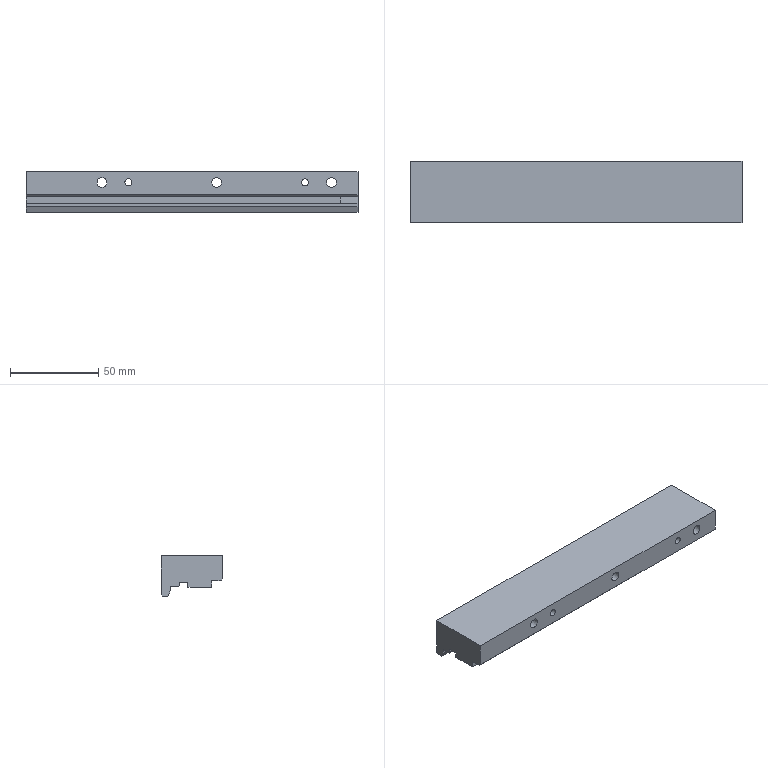Part | NX | 1 solid | 30 faces | box 188 x 35 x 22.9 mm | volume 110180 mm3 | plane 22 | cylinder 8 | commonest cylinder face diameters 5.5 x3 10 x3 4 x2
STEP:
#1=CARTESIAN_POINT('',(-94.,2.3,-17.9));
#2=VERTEX_POINT('',#1);
#3=CARTESIAN_POINT('',(-94.,-11.14,-17.9));
#4=VERTEX_POINT('',#3);
#5=CARTESIAN_POINT('',(-94.,17.5,-17.9));
#6=DIRECTION('',(0.,-1.,0.));
#7=VECTOR('',#6,1000.);
#8=LINE('',#5,#7);
#9=EDGE_CURVE('',#2,#4,#8,.T.);
#10=ORIENTED_EDGE('',*,*,#9,.F.);
#11=CARTESIAN_POINT('',(94.,2.3,-17.9));
#12=VERTEX_POINT('',#11);
#13=CARTESIAN_POINT('',(-1491.,2.3,-17.9));
#14=DIRECTION('',(1.,0.,0.));
#15=VECTOR('',#14,1000.);
#16=LINE('',#13,#15);
#17=EDGE_CURVE('',#2,#12,#16,.T.);
#18=ORIENTED_EDGE('',*,*,#17,.T.);
#19=CARTESIAN_POINT('',(94.,-9.377,-17.9));
#20=VERTEX_POINT('',#19);
#21=CARTESIAN_POINT('',(94.,17.5,-17.9));
#22=DIRECTION('',(0.,-1.,0.));
#23=VECTOR('',#22,1000.);
#24=LINE('',#21,#23);
#25=EDGE_CURVE('',#12,#20,#24,.T.);
#26=ORIENTED_EDGE('',*,*,#25,.T.);
#27=CARTESIAN_POINT('',(84.,-11.14,-17.9));
#28=VERTEX_POINT('',#27);
#29=CARTESIAN_POINT('',(84.,-11.14,-17.9));
#30=DIRECTION('',(-0.9848,-0.1736,0.));
#31=VECTOR('',#30,1000.);
#32=LINE('',#29,#31);
#33=EDGE_CURVE('',#20,#28,#32,.T.);
#34=ORIENTED_EDGE('',*,*,#33,.T.);
#35=CARTESIAN_POINT('',(-1491.,-11.14,-17.9));
#36=DIRECTION('',(1.,0.,0.));
#37=VECTOR('',#36,1000.);
#38=LINE('',#35,#37);
#39=EDGE_CURVE('',#4,#28,#38,.T.);
#40=ORIENTED_EDGE('',*,*,#39,.F.);
#41=EDGE_LOOP('',(#10,#18,#26,#34,#40));
#42=FACE_BOUND('',#41,.T.);
#43=CARTESIAN_POINT('',(94.,17.5,-17.9));
#44=DIRECTION('',(0.,0.,1.));
#45=DIRECTION('',(-1.,0.,0.));
#46=AXIS2_PLACEMENT_3D('',#43,#44,#45);
#47=PLANE('',#46);
#48=ADVANCED_FACE('',(#42),#47,.F.);
#49=CARTESIAN_POINT('',(-94.,-17.5,0.));
#50=VERTEX_POINT('',#49);
#51=CARTESIAN_POINT('',(-94.,17.5,0.));
#52=VERTEX_POINT('',#51);
#53=CARTESIAN_POINT('',(-94.,17.5,0.));
#54=DIRECTION('',(0.,1.,0.));
#55=VECTOR('',#54,1000.);
#56=LINE('',#53,#55);
#57=EDGE_CURVE('',#50,#52,#56,.T.);
#58=ORIENTED_EDGE('',*,*,#57,.F.);
#59=CARTESIAN_POINT('',(94.,-17.5,0.));
#60=VERTEX_POINT('',#59);
#61=CARTESIAN_POINT('',(94.,-17.5,0.));
#62=DIRECTION('',(1.,0.,0.));
#63=VECTOR('',#62,1000.);
#64=LINE('',#61,#63);
#65=EDGE_CURVE('',#50,#60,#64,.T.);
#66=ORIENTED_EDGE('',*,*,#65,.T.);
#67=CARTESIAN_POINT('',(94.,17.5,0.));
#68=VERTEX_POINT('',#67);
#69=CARTESIAN_POINT('',(94.,17.5,0.));
#70=DIRECTION('',(0.,-1.,0.));
#71=VECTOR('',#70,1000.);
#72=LINE('',#69,#71);
#73=EDGE_CURVE('',#68,#60,#72,.T.);
#74=ORIENTED_EDGE('',*,*,#73,.F.);
#75=CARTESIAN_POINT('',(94.,17.5,0.));
#76=DIRECTION('',(1.,0.,0.));
#77=VECTOR('',#76,1000.);
#78=LINE('',#75,#77);
#79=EDGE_CURVE('',#52,#68,#78,.T.);
#80=ORIENTED_EDGE('',*,*,#79,.F.);
#81=EDGE_LOOP('',(#58,#66,#74,#80));
#82=FACE_BOUND('',#81,.T.);
#83=CARTESIAN_POINT('',(94.,17.5,0.));
#84=DIRECTION('',(0.,0.,-1.));
#85=DIRECTION('',(1.,0.,0.));
#86=AXIS2_PLACEMENT_3D('',#83,#84,#85);
#87=PLANE('',#86);
#88=ADVANCED_FACE('',(#82),#87,.F.);
#89=CARTESIAN_POINT('',(-36.,17.5,-8.));
#90=VERTEX_POINT('',#89);
#91=CARTESIAN_POINT('',(-36.,17.5,-6.));
#92=DIRECTION('',(0.,1.,0.));
#93=DIRECTION('',(0.,0.,-1.));
#94=AXIS2_PLACEMENT_3D('',#91,#92,#93);
#95=CIRCLE('',#94,2.);
#96=EDGE_CURVE('',#90,#90,#95,.T.);
#97=ORIENTED_EDGE('',*,*,#96,.F.);
#98=EDGE_LOOP('',(#97));
#99=FACE_BOUND('',#98,.T.);
#100=CARTESIAN_POINT('',(64.,17.5,-8.));
#101=VERTEX_POINT('',#100);
#102=CARTESIAN_POINT('',(64.,17.5,-6.));
#103=DIRECTION('',(0.,1.,0.));
#104=DIRECTION('',(0.,0.,-1.));
#105=AXIS2_PLACEMENT_3D('',#102,#103,#104);
#106=CIRCLE('',#105,2.);
#107=EDGE_CURVE('',#101,#101,#106,.T.);
#108=ORIENTED_EDGE('',*,*,#107,.F.);
#109=EDGE_LOOP('',(#108));
#110=FACE_BOUND('',#109,.T.);
#111=CARTESIAN_POINT('',(79.,17.5,-11.));
#112=VERTEX_POINT('',#111);
#113=CARTESIAN_POINT('',(79.,17.5,-6.));
#114=DIRECTION('',(0.,1.,0.));
#115=DIRECTION('',(0.,0.,-1.));
#116=AXIS2_PLACEMENT_3D('',#113,#114,#115);
#117=CIRCLE('',#116,5.);
#118=EDGE_CURVE('',#112,#112,#117,.T.);
#119=ORIENTED_EDGE('',*,*,#118,.F.);
#120=EDGE_LOOP('',(#119));
#121=FACE_BOUND('',#120,.T.);
#122=CARTESIAN_POINT('',(-51.,17.5,-11.));
#123=VERTEX_POINT('',#122);
#124=CARTESIAN_POINT('',(-51.,17.5,-6.));
#125=DIRECTION('',(0.,1.,0.));
#126=DIRECTION('',(0.,0.,-1.));
#127=AXIS2_PLACEMENT_3D('',#124,#125,#126);
#128=CIRCLE('',#127,5.);
#129=EDGE_CURVE('',#123,#123,#128,.T.);
#130=ORIENTED_EDGE('',*,*,#129,.F.);
#131=EDGE_LOOP('',(#130));
#132=FACE_BOUND('',#131,.T.);
#133=CARTESIAN_POINT('',(14.,17.5,-11.));
#134=VERTEX_POINT('',#133);
#135=CARTESIAN_POINT('',(14.,17.5,-6.));
#136=DIRECTION('',(0.,1.,0.));
#137=DIRECTION('',(0.,0.,-1.));
#138=AXIS2_PLACEMENT_3D('',#135,#136,#137);
#139=CIRCLE('',#138,5.);
#140=EDGE_CURVE('',#134,#134,#139,.T.);
#141=ORIENTED_EDGE('',*,*,#140,.F.);
#142=EDGE_LOOP('',(#141));
#143=FACE_BOUND('',#142,.T.);
#144=CARTESIAN_POINT('',(94.,17.5,-21.9));
#145=VERTEX_POINT('',#144);
#146=CARTESIAN_POINT('',(-94.,17.5,-21.9));
#147=VERTEX_POINT('',#146);
#148=CARTESIAN_POINT('',(94.,17.5,-21.9));
#149=DIRECTION('',(-1.,0.,0.));
#150=VECTOR('',#149,1000.);
#151=LINE('',#148,#150);
#152=EDGE_CURVE('',#145,#147,#151,.T.);
#153=ORIENTED_EDGE('',*,*,#152,.T.);
#154=CARTESIAN_POINT('',(-94.,17.5,-17.9));
#155=DIRECTION('',(0.,0.,1.));
#156=VECTOR('',#155,1000.);
#157=LINE('',#154,#156);
#158=EDGE_CURVE('',#147,#52,#157,.T.);
#159=ORIENTED_EDGE('',*,*,#158,.T.);
#160=ORIENTED_EDGE('',*,*,#79,.T.);
#161=CARTESIAN_POINT('',(94.,17.5,0.));
#162=DIRECTION('',(0.,0.,-1.));
#163=VECTOR('',#162,1000.);
#164=LINE('',#161,#163);
#165=EDGE_CURVE('',#68,#145,#164,.T.);
#166=ORIENTED_EDGE('',*,*,#165,.T.);
#167=EDGE_LOOP('',(#153,#159,#160,#166));
#168=FACE_BOUND('',#167,.T.);
#169=CARTESIAN_POINT('',(94.,17.5,-17.9));
#170=DIRECTION('',(0.,1.,0.));
#171=DIRECTION('',(0.,0.,1.));
#172=AXIS2_PLACEMENT_3D('',#169,#170,#171);
#173=PLANE('',#172);
#174=ADVANCED_FACE('',(#99,#110,#121,#132,#143,#168),#173,.T.);
#175=CARTESIAN_POINT('',(-36.,-17.5,-8.));
#176=VERTEX_POINT('',#175);
#177=CARTESIAN_POINT('',(-36.,-17.5,-6.));
#178=DIRECTION('',(0.,1.,0.));
#179=DIRECTION('',(0.,0.,-1.));
#180=AXIS2_PLACEMENT_3D('',#177,#178,#179);
#181=CIRCLE('',#180,2.);
#182=EDGE_CURVE('',#176,#176,#181,.T.);
#183=ORIENTED_EDGE('',*,*,#182,.T.);
#184=EDGE_LOOP('',(#183));
#185=FACE_BOUND('',#184,.T.);
#186=CARTESIAN_POINT('',(64.,-17.5,-8.));
#187=VERTEX_POINT('',#186);
#188=CARTESIAN_POINT('',(64.,-17.5,-6.));
#189=DIRECTION('',(0.,1.,0.));
#190=DIRECTION('',(0.,0.,-1.));
#191=AXIS2_PLACEMENT_3D('',#188,#189,#190);
#192=CIRCLE('',#191,2.);
#193=EDGE_CURVE('',#187,#187,#192,.T.);
#194=ORIENTED_EDGE('',*,*,#193,.T.);
#195=EDGE_LOOP('',(#194));
#196=FACE_BOUND('',#195,.T.);
#197=CARTESIAN_POINT('',(79.,-17.5,-8.75));
#198=VERTEX_POINT('',#197);
#199=CARTESIAN_POINT('',(79.,-17.5,-6.));
#200=DIRECTION('',(0.,1.,0.));
#201=DIRECTION('',(0.,0.,-1.));
#202=AXIS2_PLACEMENT_3D('',#199,#200,#201);
#203=CIRCLE('',#202,2.75);
#204=EDGE_CURVE('',#198,#198,#203,.T.);
#205=ORIENTED_EDGE('',*,*,#204,.T.);
#206=EDGE_LOOP('',(#205));
#207=FACE_BOUND('',#206,.T.);
#208=CARTESIAN_POINT('',(-51.,-17.5,-8.75));
#209=VERTEX_POINT('',#208);
#210=CARTESIAN_POINT('',(-51.,-17.5,-6.));
#211=DIRECTION('',(0.,1.,0.));
#212=DIRECTION('',(0.,0.,-1.));
#213=AXIS2_PLACEMENT_3D('',#210,#211,#212);
#214=CIRCLE('',#213,2.75);
#215=EDGE_CURVE('',#209,#209,#214,.T.);
#216=ORIENTED_EDGE('',*,*,#215,.T.);
#217=EDGE_LOOP('',(#216));
#218=FACE_BOUND('',#217,.T.);
#219=CARTESIAN_POINT('',(14.,-17.5,-8.75));
#220=VERTEX_POINT('',#219);
#221=CARTESIAN_POINT('',(14.,-17.5,-6.));
#222=DIRECTION('',(0.,1.,0.));
#223=DIRECTION('',(0.,0.,-1.));
#224=AXIS2_PLACEMENT_3D('',#221,#222,#223);
#225=CIRCLE('',#224,2.75);
#226=EDGE_CURVE('',#220,#220,#225,.T.);
#227=ORIENTED_EDGE('',*,*,#226,.T.);
#228=EDGE_LOOP('',(#227));
#229=FACE_BOUND('',#228,.T.);
#230=CARTESIAN_POINT('',(-94.,-17.5,-13.1));
#231=VERTEX_POINT('',#230);
#232=CARTESIAN_POINT('',(-94.,-17.5,-17.9));
#233=DIRECTION('',(0.,0.,1.));
#234=VECTOR('',#233,1000.);
#235=LINE('',#232,#234);
#236=EDGE_CURVE('',#231,#50,#235,.T.);
#237=ORIENTED_EDGE('',*,*,#236,.F.);
#238=CARTESIAN_POINT('',(94.,-17.5,-13.1));
#239=VERTEX_POINT('',#238);
#240=CARTESIAN_POINT('',(94.,-17.5,-13.1));
#241=DIRECTION('',(1.,0.,0.));
#242=VECTOR('',#241,1000.);
#243=LINE('',#240,#242);
#244=EDGE_CURVE('',#231,#239,#243,.T.);
#245=ORIENTED_EDGE('',*,*,#244,.T.);
#246=CARTESIAN_POINT('',(94.,-17.5,0.));
#247=DIRECTION('',(0.,0.,-1.));
#248=VECTOR('',#247,1000.);
#249=LINE('',#246,#248);
#250=EDGE_CURVE('',#60,#239,#249,.T.);
#251=ORIENTED_EDGE('',*,*,#250,.F.);
#252=ORIENTED_EDGE('',*,*,#65,.F.);
#253=EDGE_LOOP('',(#237,#245,#251,#252));
#254=FACE_BOUND('',#253,.T.);
#255=CARTESIAN_POINT('',(94.,-17.5,-17.9));
#256=DIRECTION('',(0.,1.,0.));
#257=DIRECTION('',(0.,0.,1.));
#258=AXIS2_PLACEMENT_3D('',#255,#256,#257);
#259=PLANE('',#258);
#260=ADVANCED_FACE('',(#185,#196,#207,#218,#229,#254),#259,.F.);
#261=CARTESIAN_POINT('',(-94.,2.3,-14.9));
#262=VERTEX_POINT('',#261);
#263=CARTESIAN_POINT('',(-94.,2.3,-17.9));
#264=DIRECTION('',(0.,0.,-1.));
#265=VECTOR('',#264,1000.);
#266=LINE('',#263,#265);
#267=EDGE_CURVE('',#262,#2,#266,.T.);
#268=ORIENTED_EDGE('',*,*,#267,.F.);
#269=CARTESIAN_POINT('',(94.,2.3,-14.9));
#270=VERTEX_POINT('',#269);
#271=CARTESIAN_POINT('',(-1491.,2.3,-14.9));
#272=DIRECTION('',(1.,0.,0.));
#273=VECTOR('',#272,1000.);
#274=LINE('',#271,#273);
#275=EDGE_CURVE('',#262,#270,#274,.T.);
#276=ORIENTED_EDGE('',*,*,#275,.T.);
#277=CARTESIAN_POINT('',(94.,2.3,-17.9));
#278=DIRECTION('',(0.,0.,-1.));
#279=VECTOR('',#278,1000.);
#280=LINE('',#277,#279);
#281=EDGE_CURVE('',#270,#12,#280,.T.);
#282=ORIENTED_EDGE('',*,*,#281,.T.);
#283=ORIENTED_EDGE('',*,*,#17,.F.);
#284=EDGE_LOOP('',(#268,#276,#282,#283));
#285=FACE_BOUND('',#284,.T.);
#286=CARTESIAN_POINT('',(-1491.,2.3,-17.9));
#287=DIRECTION('',(0.,-1.,0.));
#288=DIRECTION('',(0.,0.,-1.));
#289=AXIS2_PLACEMENT_3D('',#286,#287,#288);
#290=PLANE('',#289);
#291=ADVANCED_FACE('',(#285),#290,.F.);
#292=CARTESIAN_POINT('',(-94.,7.3,-14.9));
#293=VERTEX_POINT('',#292);
#294=CARTESIAN_POINT('',(-94.,2.3,-14.9));
#295=DIRECTION('',(0.,-1.,0.));
#296=VECTOR('',#295,1000.);
#297=LINE('',#294,#296);
#298=EDGE_CURVE('',#293,#262,#297,.T.);
#299=ORIENTED_EDGE('',*,*,#298,.F.);
#300=CARTESIAN_POINT('',(94.,7.3,-14.9));
#301=VERTEX_POINT('',#300);
#302=CARTESIAN_POINT('',(-1491.,7.3,-14.9));
#303=DIRECTION('',(1.,0.,0.));
#304=VECTOR('',#303,1000.);
#305=LINE('',#302,#304);
#306=EDGE_CURVE('',#293,#301,#305,.T.);
#307=ORIENTED_EDGE('',*,*,#306,.T.);
#308=CARTESIAN_POINT('',(94.,2.3,-14.9));
#309=DIRECTION('',(0.,-1.,0.));
#310=VECTOR('',#309,1000.);
#311=LINE('',#308,#310);
#312=EDGE_CURVE('',#301,#270,#311,.T.);
#313=ORIENTED_EDGE('',*,*,#312,.T.);
#314=ORIENTED_EDGE('',*,*,#275,.F.);
#315=EDGE_LOOP('',(#299,#307,#313,#314));
#316=FACE_BOUND('',#315,.T.);
#317=CARTESIAN_POINT('',(-1491.,2.3,-14.9));
#318=DIRECTION('',(0.,0.,1.));
#319=DIRECTION('',(-1.,0.,0.));
#320=AXIS2_PLACEMENT_3D('',#317,#318,#319);
#321=PLANE('',#320);
#322=ADVANCED_FACE('',(#316),#321,.F.);
#323=CARTESIAN_POINT('',(-94.,7.3,-17.04));
#324=VERTEX_POINT('',#323);
#325=CARTESIAN_POINT('',(-94.,7.3,-14.9));
#326=DIRECTION('',(0.,0.,1.));
#327=VECTOR('',#326,1000.);
#328=LINE('',#325,#327);
#329=EDGE_CURVE('',#324,#293,#328,.T.);
#330=ORIENTED_EDGE('',*,*,#329,.F.);
#331=CARTESIAN_POINT('',(94.,7.3,-17.04));
#332=VERTEX_POINT('',#331);
#333=CARTESIAN_POINT('',(-1491.,7.3,-17.04));
#334=DIRECTION('',(1.,0.,0.));
#335=VECTOR('',#334,1000.);
#336=LINE('',#333,#335);
#337=EDGE_CURVE('',#324,#332,#336,.T.);
#338=ORIENTED_EDGE('',*,*,#337,.T.);
#339=CARTESIAN_POINT('',(94.,7.3,-14.9));
#340=DIRECTION('',(0.,0.,1.));
#341=VECTOR('',#340,1000.);
#342=LINE('',#339,#341);
#343=EDGE_CURVE('',#332,#301,#342,.T.);
#344=ORIENTED_EDGE('',*,*,#343,.T.);
#345=ORIENTED_EDGE('',*,*,#306,.F.);
#346=EDGE_LOOP('',(#330,#338,#344,#345));
#347=FACE_BOUND('',#346,.T.);
#348=CARTESIAN_POINT('',(-1491.,7.3,-14.9));
#349=DIRECTION('',(0.,1.,0.));
#350=DIRECTION('',(0.,0.,1.));
#351=AXIS2_PLACEMENT_3D('',#348,#349,#350);
#352=PLANE('',#351);
#353=ADVANCED_FACE('',(#347),#352,.F.);
#354=CARTESIAN_POINT('',(-94.,12.2,-17.54));
#355=VERTEX_POINT('',#354);
#356=CARTESIAN_POINT('',(-94.,7.533,-17.54));
#357=VERTEX_POINT('',#356);
#358=CARTESIAN_POINT('',(-94.,7.3,-17.54));
#359=DIRECTION('',(0.,-1.,0.));
#360=VECTOR('',#359,1000.);
#361=LINE('',#358,#360);
#362=EDGE_CURVE('',#355,#357,#361,.T.);
#363=ORIENTED_EDGE('',*,*,#362,.F.);
#364=CARTESIAN_POINT('',(94.,12.2,-17.54));
#365=VERTEX_POINT('',#364);
#366=CARTESIAN_POINT('',(-1491.,12.2,-17.54));
#367=DIRECTION('',(1.,0.,0.));
#368=VECTOR('',#367,1000.);
#369=LINE('',#366,#368);
#370=EDGE_CURVE('',#355,#365,#369,.T.);
#371=ORIENTED_EDGE('',*,*,#370,.T.);
#372=CARTESIAN_POINT('',(94.,7.533,-17.54));
#373=VERTEX_POINT('',#372);
#374=CARTESIAN_POINT('',(94.,7.3,-17.54));
#375=DIRECTION('',(0.,-1.,0.));
#376=VECTOR('',#375,1000.);
#377=LINE('',#374,#376);
#378=EDGE_CURVE('',#365,#373,#377,.T.);
#379=ORIENTED_EDGE('',*,*,#378,.T.);
#380=CARTESIAN_POINT('',(-1491.,7.533,-17.54));
#381=DIRECTION('',(-1.,0.,0.));
#382=VECTOR('',#381,1000.);
#383=LINE('',#380,#382);
#384=EDGE_CURVE('',#373,#357,#383,.T.);
#385=ORIENTED_EDGE('',*,*,#384,.T.);
#386=EDGE_LOOP('',(#363,#371,#379,#385));
#387=FACE_BOUND('',#386,.T.);
#388=CARTESIAN_POINT('',(-1491.,7.3,-17.54));
#389=DIRECTION('',(0.,0.,1.));
#390=DIRECTION('',(-1.,0.,0.));
#391=AXIS2_PLACEMENT_3D('',#388,#389,#390);
#392=PLANE('',#391);
#393=ADVANCED_FACE('',(#387),#392,.F.);
#394=CARTESIAN_POINT('',(-94.,12.2,-19.9));
#395=VERTEX_POINT('',#394);
#396=CARTESIAN_POINT('',(-94.,12.2,-17.54));
#397=DIRECTION('',(0.,0.,1.));
#398=VECTOR('',#397,1000.);
#399=LINE('',#396,#398);
#400=EDGE_CURVE('',#395,#355,#399,.T.);
#401=ORIENTED_EDGE('',*,*,#400,.F.);
#402=CARTESIAN_POINT('',(94.,12.2,-19.9));
#403=VERTEX_POINT('',#402);
#404=CARTESIAN_POINT('',(94.,12.2,-19.9));
#405=DIRECTION('',(1.,0.,0.));
#406=VECTOR('',#405,1000.);
#407=LINE('',#404,#406);
#408=EDGE_CURVE('',#395,#403,#407,.T.);
#409=ORIENTED_EDGE('',*,*,#408,.T.);
#410=CARTESIAN_POINT('',(94.,12.2,-17.54));
#411=DIRECTION('',(0.,0.,1.));
#412=VECTOR('',#411,1000.);
#413=LINE('',#410,#412);
#414=EDGE_CURVE('',#403,#365,#413,.T.);
#415=ORIENTED_EDGE('',*,*,#414,.T.);
#416=ORIENTED_EDGE('',*,*,#370,.F.);
#417=EDGE_LOOP('',(#401,#409,#415,#416));
#418=FACE_BOUND('',#417,.T.);
#419=CARTESIAN_POINT('',(-1491.,12.2,-17.54));
#420=DIRECTION('',(0.,1.,0.));
#421=DIRECTION('',(0.,0.,1.));
#422=AXIS2_PLACEMENT_3D('',#419,#420,#421);
#423=PLANE('',#422);
#424=ADVANCED_FACE('',(#418),#423,.F.);
#425=ORIENTED_EDGE('',*,*,#337,.F.);
#426=CARTESIAN_POINT('',(-94.,7.3,-17.04));
#427=DIRECTION('',(0.,0.4226,-0.9063));
#428=VECTOR('',#427,1000.);
#429=LINE('',#426,#428);
#430=EDGE_CURVE('',#324,#357,#429,.T.);
#431=ORIENTED_EDGE('',*,*,#430,.T.);
#432=ORIENTED_EDGE('',*,*,#384,.F.);
#433=CARTESIAN_POINT('',(94.,7.3,-17.04));
#434=DIRECTION('',(0.,0.4226,-0.9063));
#435=VECTOR('',#434,1000.);
#436=LINE('',#433,#435);
#437=EDGE_CURVE('',#332,#373,#436,.T.);
#438=ORIENTED_EDGE('',*,*,#437,.F.);
#439=EDGE_LOOP('',(#425,#431,#432,#438));
#440=FACE_BOUND('',#439,.T.);
#441=CARTESIAN_POINT('',(-1491.,7.3,-17.04));
#442=DIRECTION('',(0.,0.9063,0.4226));
#443=DIRECTION('',(-1.,0.,0.));
#444=AXIS2_PLACEMENT_3D('',#441,#442,#443);
#445=PLANE('',#444);
#446=ADVANCED_FACE('',(#440),#445,.F.);
#447=CARTESIAN_POINT('',(-94.,-11.14,-14.1));
#448=VERTEX_POINT('',#447);
#449=CARTESIAN_POINT('',(-94.,-16.5,-14.1));
#450=VERTEX_POINT('',#449);
#451=CARTESIAN_POINT('',(-94.,-17.5,-14.1));
#452=DIRECTION('',(0.,-1.,0.));
#453=VECTOR('',#452,1000.);
#454=LINE('',#451,#453);
#455=EDGE_CURVE('',#448,#450,#454,.T.);
#456=ORIENTED_EDGE('',*,*,#455,.F.);
#457=CARTESIAN_POINT('',(84.,-11.14,-14.1));
#458=VERTEX_POINT('',#457);
#459=CARTESIAN_POINT('',(-1491.,-11.14,-14.1));
#460=DIRECTION('',(1.,0.,0.));
#461=VECTOR('',#460,1000.);
#462=LINE('',#459,#461);
#463=EDGE_CURVE('',#448,#458,#462,.T.);
#464=ORIENTED_EDGE('',*,*,#463,.T.);
#465=CARTESIAN_POINT('',(94.,-9.377,-14.1));
#466=VERTEX_POINT('',#465);
#467=CARTESIAN_POINT('',(-1444.596,-280.673,-14.1));
#468=DIRECTION('',(0.9848,0.1736,0.));
#469=VECTOR('',#468,1000.);
#470=LINE('',#467,#469);
#471=EDGE_CURVE('',#458,#466,#470,.T.);
#472=ORIENTED_EDGE('',*,*,#471,.T.);
#473=CARTESIAN_POINT('',(94.,-16.5,-14.1));
#474=VERTEX_POINT('',#473);
#475=CARTESIAN_POINT('',(94.,-17.5,-14.1));
#476=DIRECTION('',(0.,-1.,0.));
#477=VECTOR('',#476,1000.);
#478=LINE('',#475,#477);
#479=EDGE_CURVE('',#466,#474,#478,.T.);
#480=ORIENTED_EDGE('',*,*,#479,.T.);
#481=CARTESIAN_POINT('',(-1491.,-16.5,-14.1));
#482=DIRECTION('',(-1.,0.,0.));
#483=VECTOR('',#482,1000.);
#484=LINE('',#481,#483);
#485=EDGE_CURVE('',#474,#450,#484,.T.);
#486=ORIENTED_EDGE('',*,*,#485,.T.);
#487=EDGE_LOOP('',(#456,#464,#472,#480,#486));
#488=FACE_BOUND('',#487,.T.);
#489=CARTESIAN_POINT('',(-1491.,-17.5,-14.1));
#490=DIRECTION('',(0.,0.,1.));
#491=DIRECTION('',(-1.,0.,0.));
#492=AXIS2_PLACEMENT_3D('',#489,#490,#491);
#493=PLANE('',#492);
#494=ADVANCED_FACE('',(#488),#493,.F.);
#495=CARTESIAN_POINT('',(-94.,-11.14,-14.1));
#496=DIRECTION('',(0.,0.,1.));
#497=VECTOR('',#496,1000.);
#498=LINE('',#495,#497);
#499=EDGE_CURVE('',#4,#448,#498,.T.);
#500=ORIENTED_EDGE('',*,*,#499,.F.);
#501=ORIENTED_EDGE('',*,*,#39,.T.);
#502=CARTESIAN_POINT('',(84.,-11.14,-14.1));
#503=DIRECTION('',(0.,0.,1.));
#504=VECTOR('',#503,1000.);
#505=LINE('',#502,#504);
#506=EDGE_CURVE('',#28,#458,#505,.T.);
#507=ORIENTED_EDGE('',*,*,#506,.T.);
#508=ORIENTED_EDGE('',*,*,#463,.F.);
#509=EDGE_LOOP('',(#500,#501,#507,#508));
#510=FACE_BOUND('',#509,.T.);
#511=CARTESIAN_POINT('',(-1491.,-11.14,-14.1));
#512=DIRECTION('',(0.,1.,0.));
#513=DIRECTION('',(0.,0.,1.));
#514=AXIS2_PLACEMENT_3D('',#511,#512,#513);
#515=PLANE('',#514);
#516=ADVANCED_FACE('',(#510),#515,.F.);
#517=ORIENTED_EDGE('',*,*,#244,.F.);
#518=CARTESIAN_POINT('',(-94.,-17.5,-13.1));
#519=DIRECTION('',(0.,0.7071,-0.7071));
#520=VECTOR('',#519,1000.);
#521=LINE('',#518,#520);
#522=EDGE_CURVE('',#231,#450,#521,.T.);
#523=ORIENTED_EDGE('',*,*,#522,.T.);
#524=ORIENTED_EDGE('',*,*,#485,.F.);
#525=CARTESIAN_POINT('',(94.,-17.5,-13.1));
#526=DIRECTION('',(0.,0.7071,-0.7071));
#527=VECTOR('',#526,1000.);
#528=LINE('',#525,#527);
#529=EDGE_CURVE('',#239,#474,#528,.T.);
#530=ORIENTED_EDGE('',*,*,#529,.F.);
#531=EDGE_LOOP('',(#517,#523,#524,#530));
#532=FACE_BOUND('',#531,.T.);
#533=CARTESIAN_POINT('',(94.,-17.5,-13.1));
#534=DIRECTION('',(0.,0.7071,0.7071));
#535=DIRECTION('',(-1.,0.,0.));
#536=AXIS2_PLACEMENT_3D('',#533,#534,#535);
#537=PLANE('',#536);
#538=ADVANCED_FACE('',(#532),#537,.F.);
#539=CARTESIAN_POINT('',(94.,13.599,-22.9));
#540=VERTEX_POINT('',#539);
#541=CARTESIAN_POINT('',(-94.,13.599,-22.9));
#542=VERTEX_POINT('',#541);
#543=CARTESIAN_POINT('',(-1491.,13.599,-22.9));
#544=DIRECTION('',(-1.,0.,0.));
#545=VECTOR('',#544,1000.);
#546=LINE('',#543,#545);
#547=EDGE_CURVE('',#540,#542,#546,.T.);
#548=ORIENTED_EDGE('',*,*,#547,.T.);
#549=CARTESIAN_POINT('',(-94.,16.5,-22.9));
#550=VERTEX_POINT('',#549);
#551=CARTESIAN_POINT('',(-94.,0.,-22.9));
#552=DIRECTION('',(0.,1.,0.));
#553=VECTOR('',#552,1000.);
#554=LINE('',#551,#553);
#555=EDGE_CURVE('',#542,#550,#554,.T.);
#556=ORIENTED_EDGE('',*,*,#555,.T.);
#557=CARTESIAN_POINT('',(94.,16.5,-22.9));
#558=VERTEX_POINT('',#557);
#559=CARTESIAN_POINT('',(-698.5,16.5,-22.9));
#560=DIRECTION('',(1.,0.,0.));
#561=VECTOR('',#560,1000.);
#562=LINE('',#559,#561);
#563=EDGE_CURVE('',#550,#558,#562,.T.);
#564=ORIENTED_EDGE('',*,*,#563,.T.);
#565=CARTESIAN_POINT('',(94.,17.5,-22.9));
#566=DIRECTION('',(0.,-1.,0.));
#567=VECTOR('',#566,1000.);
#568=LINE('',#565,#567);
#569=EDGE_CURVE('',#558,#540,#568,.T.);
#570=ORIENTED_EDGE('',*,*,#569,.T.);
#571=EDGE_LOOP('',(#548,#556,#564,#570));
#572=FACE_BOUND('',#571,.T.);
#573=CARTESIAN_POINT('',(-698.5,0.,-22.9));
#574=DIRECTION('',(0.,0.,-1.));
#575=DIRECTION('',(1.,0.,0.));
#576=AXIS2_PLACEMENT_3D('',#573,#574,#575);
#577=PLANE('',#576);
#578=ADVANCED_FACE('',(#572),#577,.T.);
#579=ORIENTED_EDGE('',*,*,#408,.F.);
#580=CARTESIAN_POINT('',(-94.,13.599,-22.9));
#581=DIRECTION('',(0.,0.4226,-0.9063));
#582=VECTOR('',#581,1000.);
#583=LINE('',#580,#582);
#584=EDGE_CURVE('',#395,#542,#583,.T.);
#585=ORIENTED_EDGE('',*,*,#584,.T.);
#586=ORIENTED_EDGE('',*,*,#547,.F.);
#587=CARTESIAN_POINT('',(94.,13.599,-22.9));
#588=DIRECTION('',(0.,0.4226,-0.9063));
#589=VECTOR('',#588,1000.);
#590=LINE('',#587,#589);
#591=EDGE_CURVE('',#403,#540,#590,.T.);
#592=ORIENTED_EDGE('',*,*,#591,.F.);
#593=EDGE_LOOP('',(#579,#585,#586,#592));
#594=FACE_BOUND('',#593,.T.);
#595=CARTESIAN_POINT('',(-698.5,13.599,-22.9));
#596=DIRECTION('',(0.,-0.9063,-0.4226));
#597=DIRECTION('',(-1.,0.,0.));
#598=AXIS2_PLACEMENT_3D('',#595,#596,#597);
#599=PLANE('',#598);
#600=ADVANCED_FACE('',(#594),#599,.T.);
#601=ORIENTED_EDGE('',*,*,#563,.F.);
#602=CARTESIAN_POINT('',(-94.,16.5,-22.9));
#603=DIRECTION('',(0.,0.7071,0.7071));
#604=VECTOR('',#603,1000.);
#605=LINE('',#602,#604);
#606=EDGE_CURVE('',#550,#147,#605,.T.);
#607=ORIENTED_EDGE('',*,*,#606,.T.);
#608=ORIENTED_EDGE('',*,*,#152,.F.);
#609=CARTESIAN_POINT('',(94.,16.5,-22.9));
#610=DIRECTION('',(0.,0.7071,0.7071));
#611=VECTOR('',#610,1000.);
#612=LINE('',#609,#611);
#613=EDGE_CURVE('',#558,#145,#612,.T.);
#614=ORIENTED_EDGE('',*,*,#613,.F.);
#615=EDGE_LOOP('',(#601,#607,#608,#614));
#616=FACE_BOUND('',#615,.T.);
#617=CARTESIAN_POINT('',(-698.5,16.5,-22.9));
#618=DIRECTION('',(0.,-0.7071,0.7071));
#619=DIRECTION('',(-1.,0.,0.));
#620=AXIS2_PLACEMENT_3D('',#617,#618,#619);
#621=PLANE('',#620);
#622=ADVANCED_FACE('',(#616),#621,.F.);
#623=ORIENTED_EDGE('',*,*,#479,.F.);
#624=CARTESIAN_POINT('',(94.,-9.377,0.));
#625=DIRECTION('',(0.,0.,-1.));
#626=VECTOR('',#625,1000.);
#627=LINE('',#624,#626);
#628=EDGE_CURVE('',#466,#20,#627,.T.);
#629=ORIENTED_EDGE('',*,*,#628,.T.);
#630=ORIENTED_EDGE('',*,*,#25,.F.);
#631=ORIENTED_EDGE('',*,*,#281,.F.);
#632=ORIENTED_EDGE('',*,*,#312,.F.);
#633=ORIENTED_EDGE('',*,*,#343,.F.);
#634=ORIENTED_EDGE('',*,*,#437,.T.);
#635=ORIENTED_EDGE('',*,*,#378,.F.);
#636=ORIENTED_EDGE('',*,*,#414,.F.);
#637=ORIENTED_EDGE('',*,*,#591,.T.);
#638=ORIENTED_EDGE('',*,*,#569,.F.);
#639=ORIENTED_EDGE('',*,*,#613,.T.);
#640=ORIENTED_EDGE('',*,*,#165,.F.);
#641=ORIENTED_EDGE('',*,*,#73,.T.);
#642=ORIENTED_EDGE('',*,*,#250,.T.);
#643=ORIENTED_EDGE('',*,*,#529,.T.);
#644=EDGE_LOOP('',(#623,#629,#630,#631,#632,#633,#634,#635,#636,#637,#638,#639,#640,#641,#642,#643));
#645=FACE_BOUND('',#644,.T.);
#646=CARTESIAN_POINT('',(94.,17.5,0.));
#647=DIRECTION('',(-1.,0.,0.));
#648=DIRECTION('',(0.,0.,-1.));
#649=AXIS2_PLACEMENT_3D('',#646,#647,#648);
#650=PLANE('',#649);
#651=ADVANCED_FACE('',(#645),#650,.F.);
#652=ORIENTED_EDGE('',*,*,#33,.F.);
#653=ORIENTED_EDGE('',*,*,#628,.F.);
#654=ORIENTED_EDGE('',*,*,#471,.F.);
#655=ORIENTED_EDGE('',*,*,#506,.F.);
#656=EDGE_LOOP('',(#652,#653,#654,#655));
#657=FACE_BOUND('',#656,.T.);
#658=CARTESIAN_POINT('',(84.,-11.14,-14.1));
#659=DIRECTION('',(-0.1736,0.9848,0.));
#660=DIRECTION('',(0.,0.,-1.));
#661=AXIS2_PLACEMENT_3D('',#658,#659,#660);
#662=PLANE('',#661);
#663=ADVANCED_FACE('',(#657),#662,.F.);
#664=ORIENTED_EDGE('',*,*,#522,.F.);
#665=ORIENTED_EDGE('',*,*,#236,.T.);
#666=ORIENTED_EDGE('',*,*,#57,.T.);
#667=ORIENTED_EDGE('',*,*,#158,.F.);
#668=ORIENTED_EDGE('',*,*,#606,.F.);
#669=ORIENTED_EDGE('',*,*,#555,.F.);
#670=ORIENTED_EDGE('',*,*,#584,.F.);
#671=ORIENTED_EDGE('',*,*,#400,.T.);
#672=ORIENTED_EDGE('',*,*,#362,.T.);
#673=ORIENTED_EDGE('',*,*,#430,.F.);
#674=ORIENTED_EDGE('',*,*,#329,.T.);
#675=ORIENTED_EDGE('',*,*,#298,.T.);
#676=ORIENTED_EDGE('',*,*,#267,.T.);
#677=ORIENTED_EDGE('',*,*,#9,.T.);
#678=ORIENTED_EDGE('',*,*,#499,.T.);
#679=ORIENTED_EDGE('',*,*,#455,.T.);
#680=EDGE_LOOP('',(#664,#665,#666,#667,#668,#669,#670,#671,#672,#673,#674,#675,#676,#677,#678,#679));
#681=FACE_BOUND('',#680,.T.);
#682=CARTESIAN_POINT('',(-94.,17.5,-22.91));
#683=DIRECTION('',(-1.,0.,0.));
#684=DIRECTION('',(0.,0.,-1.));
#685=AXIS2_PLACEMENT_3D('',#682,#683,#684);
#686=PLANE('',#685);
#687=ADVANCED_FACE('',(#681),#686,.T.);
#688=ORIENTED_EDGE('',*,*,#226,.F.);
#689=EDGE_LOOP('',(#688));
#690=FACE_BOUND('',#689,.T.);
#691=CARTESIAN_POINT('',(14.,12.1,-8.75));
#692=VERTEX_POINT('',#691);
#693=CARTESIAN_POINT('',(14.,12.1,-6.));
#694=DIRECTION('',(0.,1.,0.));
#695=DIRECTION('',(0.,0.,-1.));
#696=AXIS2_PLACEMENT_3D('',#693,#694,#695);
#697=CIRCLE('',#696,2.75);
#698=EDGE_CURVE('',#692,#692,#697,.T.);
#699=ORIENTED_EDGE('',*,*,#698,.T.);
#700=EDGE_LOOP('',(#699));
#701=FACE_BOUND('',#700,.T.);
#702=CARTESIAN_POINT('',(14.,17.5,-6.));
#703=DIRECTION('',(0.,1.,0.));
#704=DIRECTION('',(0.,0.,1.));
#705=AXIS2_PLACEMENT_3D('',#702,#703,#704);
#706=CYLINDRICAL_SURFACE('',#705,2.75);
#707=ADVANCED_FACE('',(#690,#701),#706,.F.);
#708=ORIENTED_EDGE('',*,*,#698,.F.);
#709=EDGE_LOOP('',(#708));
#710=FACE_BOUND('',#709,.T.);
#711=CARTESIAN_POINT('',(14.,12.1,-11.));
#712=VERTEX_POINT('',#711);
#713=CARTESIAN_POINT('',(14.,12.1,-6.));
#714=DIRECTION('',(0.,1.,0.));
#715=DIRECTION('',(0.,0.,-1.));
#716=AXIS2_PLACEMENT_3D('',#713,#714,#715);
#717=CIRCLE('',#716,5.);
#718=EDGE_CURVE('',#712,#712,#717,.T.);
#719=ORIENTED_EDGE('',*,*,#718,.T.);
#720=EDGE_LOOP('',(#719));
#721=FACE_BOUND('',#720,.T.);
#722=CARTESIAN_POINT('',(11.25,12.1,-6.));
#723=DIRECTION('',(0.,-1.,0.));
#724=DIRECTION('',(0.,0.,-1.));
#725=AXIS2_PLACEMENT_3D('',#722,#723,#724);
#726=PLANE('',#725);
#727=ADVANCED_FACE('',(#710,#721),#726,.F.);
#728=ORIENTED_EDGE('',*,*,#718,.F.);
#729=EDGE_LOOP('',(#728));
#730=FACE_BOUND('',#729,.T.);
#731=ORIENTED_EDGE('',*,*,#140,.T.);
#732=EDGE_LOOP('',(#731));
#733=FACE_BOUND('',#732,.T.);
#734=CARTESIAN_POINT('',(14.,17.5,-6.));
#735=DIRECTION('',(0.,1.,0.));
#736=DIRECTION('',(0.,0.,1.));
#737=AXIS2_PLACEMENT_3D('',#734,#735,#736);
#738=CYLINDRICAL_SURFACE('',#737,5.);
#739=ADVANCED_FACE('',(#730,#733),#738,.F.);
#740=ORIENTED_EDGE('',*,*,#215,.F.);
#741=EDGE_LOOP('',(#740));
#742=FACE_BOUND('',#741,.T.);
#743=CARTESIAN_POINT('',(-51.,12.1,-8.75));
#744=VERTEX_POINT('',#743);
#745=CARTESIAN_POINT('',(-51.,12.1,-6.));
#746=DIRECTION('',(0.,1.,0.));
#747=DIRECTION('',(0.,0.,-1.));
#748=AXIS2_PLACEMENT_3D('',#745,#746,#747);
#749=CIRCLE('',#748,2.75);
#750=EDGE_CURVE('',#744,#744,#749,.T.);
#751=ORIENTED_EDGE('',*,*,#750,.T.);
#752=EDGE_LOOP('',(#751));
#753=FACE_BOUND('',#752,.T.);
#754=CARTESIAN_POINT('',(-51.,17.5,-6.));
#755=DIRECTION('',(0.,1.,0.));
#756=DIRECTION('',(0.,0.,1.));
#757=AXIS2_PLACEMENT_3D('',#754,#755,#756);
#758=CYLINDRICAL_SURFACE('',#757,2.75);
#759=ADVANCED_FACE('',(#742,#753),#758,.F.);
#760=ORIENTED_EDGE('',*,*,#750,.F.);
#761=EDGE_LOOP('',(#760));
#762=FACE_BOUND('',#761,.T.);
#763=CARTESIAN_POINT('',(-51.,12.1,-11.));
#764=VERTEX_POINT('',#763);
#765=CARTESIAN_POINT('',(-51.,12.1,-6.));
#766=DIRECTION('',(0.,1.,0.));
#767=DIRECTION('',(0.,0.,-1.));
#768=AXIS2_PLACEMENT_3D('',#765,#766,#767);
#769=CIRCLE('',#768,5.);
#770=EDGE_CURVE('',#764,#764,#769,.T.);
#771=ORIENTED_EDGE('',*,*,#770,.T.);
#772=EDGE_LOOP('',(#771));
#773=FACE_BOUND('',#772,.T.);
#774=CARTESIAN_POINT('',(-53.75,12.1,-6.));
#775=DIRECTION('',(0.,-1.,0.));
#776=DIRECTION('',(0.,0.,-1.));
#777=AXIS2_PLACEMENT_3D('',#774,#775,#776);
#778=PLANE('',#777);
#779=ADVANCED_FACE('',(#762,#773),#778,.F.);
#780=ORIENTED_EDGE('',*,*,#770,.F.);
#781=EDGE_LOOP('',(#780));
#782=FACE_BOUND('',#781,.T.);
#783=ORIENTED_EDGE('',*,*,#129,.T.);
#784=EDGE_LOOP('',(#783));
#785=FACE_BOUND('',#784,.T.);
#786=CARTESIAN_POINT('',(-51.,17.5,-6.));
#787=DIRECTION('',(0.,1.,0.));
#788=DIRECTION('',(0.,0.,1.));
#789=AXIS2_PLACEMENT_3D('',#786,#787,#788);
#790=CYLINDRICAL_SURFACE('',#789,5.);
#791=ADVANCED_FACE('',(#782,#785),#790,.F.);
#792=ORIENTED_EDGE('',*,*,#204,.F.);
#793=EDGE_LOOP('',(#792));
#794=FACE_BOUND('',#793,.T.);
#795=CARTESIAN_POINT('',(79.,12.1,-8.75));
#796=VERTEX_POINT('',#795);
#797=CARTESIAN_POINT('',(79.,12.1,-6.));
#798=DIRECTION('',(0.,1.,0.));
#799=DIRECTION('',(0.,0.,-1.));
#800=AXIS2_PLACEMENT_3D('',#797,#798,#799);
#801=CIRCLE('',#800,2.75);
#802=EDGE_CURVE('',#796,#796,#801,.T.);
#803=ORIENTED_EDGE('',*,*,#802,.T.);
#804=EDGE_LOOP('',(#803));
#805=FACE_BOUND('',#804,.T.);
#806=CARTESIAN_POINT('',(79.,17.5,-6.));
#807=DIRECTION('',(0.,1.,0.));
#808=DIRECTION('',(0.,0.,1.));
#809=AXIS2_PLACEMENT_3D('',#806,#807,#808);
#810=CYLINDRICAL_SURFACE('',#809,2.75);
#811=ADVANCED_FACE('',(#794,#805),#810,.F.);
#812=ORIENTED_EDGE('',*,*,#802,.F.);
#813=EDGE_LOOP('',(#812));
#814=FACE_BOUND('',#813,.T.);
#815=CARTESIAN_POINT('',(79.,12.1,-11.));
#816=VERTEX_POINT('',#815);
#817=CARTESIAN_POINT('',(79.,12.1,-6.));
#818=DIRECTION('',(0.,1.,0.));
#819=DIRECTION('',(0.,0.,-1.));
#820=AXIS2_PLACEMENT_3D('',#817,#818,#819);
#821=CIRCLE('',#820,5.);
#822=EDGE_CURVE('',#816,#816,#821,.T.);
#823=ORIENTED_EDGE('',*,*,#822,.T.);
#824=EDGE_LOOP('',(#823));
#825=FACE_BOUND('',#824,.T.);
#826=CARTESIAN_POINT('',(76.25,12.1,-6.));
#827=DIRECTION('',(0.,-1.,0.));
#828=DIRECTION('',(0.,0.,-1.));
#829=AXIS2_PLACEMENT_3D('',#826,#827,#828);
#830=PLANE('',#829);
#831=ADVANCED_FACE('',(#814,#825),#830,.F.);
#832=ORIENTED_EDGE('',*,*,#822,.F.);
#833=EDGE_LOOP('',(#832));
#834=FACE_BOUND('',#833,.T.);
#835=ORIENTED_EDGE('',*,*,#118,.T.);
#836=EDGE_LOOP('',(#835));
#837=FACE_BOUND('',#836,.T.);
#838=CARTESIAN_POINT('',(79.,17.5,-6.));
#839=DIRECTION('',(0.,1.,0.));
#840=DIRECTION('',(0.,0.,1.));
#841=AXIS2_PLACEMENT_3D('',#838,#839,#840);
#842=CYLINDRICAL_SURFACE('',#841,5.);
#843=ADVANCED_FACE('',(#834,#837),#842,.F.);
#844=ORIENTED_EDGE('',*,*,#193,.F.);
#845=EDGE_LOOP('',(#844));
#846=FACE_BOUND('',#845,.T.);
#847=ORIENTED_EDGE('',*,*,#107,.T.);
#848=EDGE_LOOP('',(#847));
#849=FACE_BOUND('',#848,.T.);
#850=CARTESIAN_POINT('',(64.,-17.5,-6.));
#851=DIRECTION('',(0.,1.,0.));
#852=DIRECTION('',(0.,0.,1.));
#853=AXIS2_PLACEMENT_3D('',#850,#851,#852);
#854=CYLINDRICAL_SURFACE('',#853,2.);
#855=ADVANCED_FACE('',(#846,#849),#854,.F.);
#856=ORIENTED_EDGE('',*,*,#182,.F.);
#857=EDGE_LOOP('',(#856));
#858=FACE_BOUND('',#857,.T.);
#859=ORIENTED_EDGE('',*,*,#96,.T.);
#860=EDGE_LOOP('',(#859));
#861=FACE_BOUND('',#860,.T.);
#862=CARTESIAN_POINT('',(-36.,-17.5,-6.));
#863=DIRECTION('',(0.,1.,0.));
#864=DIRECTION('',(0.,0.,1.));
#865=AXIS2_PLACEMENT_3D('',#862,#863,#864);
#866=CYLINDRICAL_SURFACE('',#865,2.);
#867=ADVANCED_FACE('',(#858,#861),#866,.F.);
#868=CLOSED_SHELL('',(#48,#88,#174,#260,#291,#322,#353,#393,#424,#446,#494,#516,#538,#578,#600,#622,#651,#663,#687,#707,#727,#739,#759,#779,#791,#811,#831,#843,#855,#867));
#869=MANIFOLD_SOLID_BREP('',#868);
#870=(LENGTH_UNIT()NAMED_UNIT(*)SI_UNIT(.MILLI.,.METRE.));
#871=UNCERTAINTY_MEASURE_WITH_UNIT(LENGTH_MEASURE(0.00001),#870,'','');
#872=(NAMED_UNIT(*)PLANE_ANGLE_UNIT()SI_UNIT($,.RADIAN.));
#873=(NAMED_UNIT(*)SI_UNIT($,.STERADIAN.)SOLID_ANGLE_UNIT());
#874=(GEOMETRIC_REPRESENTATION_CONTEXT(3)GLOBAL_UNCERTAINTY_ASSIGNED_CONTEXT((#871))GLOBAL_UNIT_ASSIGNED_CONTEXT((#870,#872,#873))REPRESENTATION_CONTEXT('',''));
#875=ADVANCED_BREP_SHAPE_REPRESENTATION('',(#869),#874);